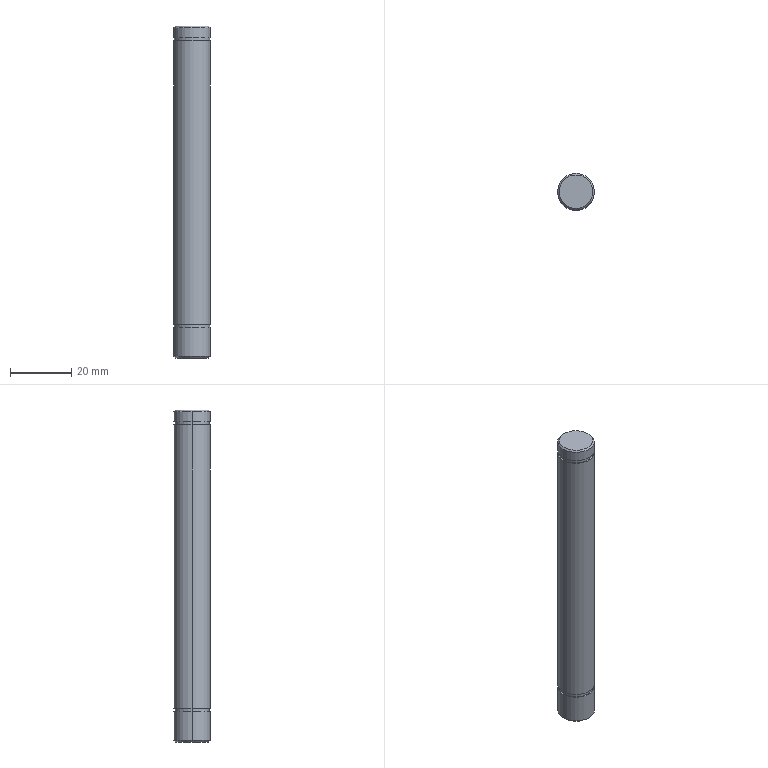Part | STEP file | 2013 Bag feed rotary shaft | 1 solid | 24 faces | box 12 x 12 x 108.5 mm | volume 11898 mm3 | cylinder 12 | cone 6 | plane 6 | commonest cylinder face diameters 12 x6 11.5 x4 5 x2
STEP:
#1=CARTESIAN_POINT('',(0.,0.,0.));
#2=DIRECTION('',(0.,0.,1.));
#3=DIRECTION('',(1.,0.,0.));
#4=AXIS2_PLACEMENT_3D('',#1,#2,#3);
#5=CARTESIAN_POINT('',(-5.5,0.,-11.1));
#6=VERTEX_POINT('',#5);
#7=CARTESIAN_POINT('',(5.5,0.,-11.1));
#8=VERTEX_POINT('',#7);
#9=CARTESIAN_POINT('',(0.,0.,-11.1));
#10=DIRECTION('',(0.,0.,-1.));
#11=DIRECTION('',(-1.,0.,0.));
#12=AXIS2_PLACEMENT_3D('',#9,#10,#11);
#13=CIRCLE('',#12,5.5);
#14=CARTESIAN_POINT('',(0.,0.,-11.1));
#15=DIRECTION('',(0.,0.,1.));
#16=DIRECTION('',(1.,0.,0.));
#17=AXIS2_PLACEMENT_3D('',#14,#15,#16);
#18=CONICAL_SURFACE('',#17,5.5,0.7854);
#19=CARTESIAN_POINT('',(3.142,0.));
#20=DIRECTION('',(-1.,0.));
#21=VECTOR('',#20,1.);
#22=LINE('',#19,#21);
#23=(GEOMETRIC_REPRESENTATION_CONTEXT(2)PARAMETRIC_REPRESENTATION_CONTEXT()REPRESENTATION_CONTEXT('',''));
#24=DEFINITIONAL_REPRESENTATION('',(#22),#23);
#25=PCURVE('',#18,#24);
#26=CARTESIAN_POINT('',(0.,0.,-11.1));
#27=DIRECTION('',(0.,0.,-1.));
#28=DIRECTION('',(-1.,0.,0.));
#29=AXIS2_PLACEMENT_3D('',#26,#27,#28);
#30=PLANE('',#29);
#31=CARTESIAN_POINT('',(0.,0.));
#32=DIRECTION('',(1.,0.));
#33=AXIS2_PLACEMENT_2D('',#31,#32);
#34=CIRCLE('',#33,5.5);
#35=(GEOMETRIC_REPRESENTATION_CONTEXT(2)PARAMETRIC_REPRESENTATION_CONTEXT()REPRESENTATION_CONTEXT('',''));
#36=DEFINITIONAL_REPRESENTATION('',(#34),#35);
#37=PCURVE('',#30,#36);
#38=SURFACE_CURVE('',#13,(#25,#37),.PCURVE_S1.);
#39=EDGE_CURVE('',#6,#8,#38,.T.);
#40=ORIENTED_EDGE('',*,*,#39,.F.);
#41=CARTESIAN_POINT('',(-6.,0.,-10.6));
#42=VERTEX_POINT('',#41);
#43=CARTESIAN_POINT('',(-5.5,0.,-11.1));
#44=DIRECTION('',(-0.7071,0.,0.7071));
#45=VECTOR('',#44,1.);
#46=LINE('',#43,#45);
#47=CARTESIAN_POINT('',(3.142,0.));
#48=DIRECTION('',(0.,1.));
#49=VECTOR('',#48,1.);
#50=LINE('',#47,#49);
#51=(GEOMETRIC_REPRESENTATION_CONTEXT(2)PARAMETRIC_REPRESENTATION_CONTEXT()REPRESENTATION_CONTEXT('',''));
#52=DEFINITIONAL_REPRESENTATION('',(#50),#51);
#53=PCURVE('',#18,#52);
#54=CARTESIAN_POINT('',(0.,0.,-11.1));
#55=DIRECTION('',(0.,0.,1.));
#56=DIRECTION('',(1.,0.,0.));
#57=AXIS2_PLACEMENT_3D('',#54,#55,#56);
#58=CONICAL_SURFACE('',#57,5.5,0.7854);
#59=CARTESIAN_POINT('',(3.142,0.));
#60=DIRECTION('',(0.,1.));
#61=VECTOR('',#60,1.);
#62=LINE('',#59,#61);
#63=(GEOMETRIC_REPRESENTATION_CONTEXT(2)PARAMETRIC_REPRESENTATION_CONTEXT()REPRESENTATION_CONTEXT('',''));
#64=DEFINITIONAL_REPRESENTATION('',(#62),#63);
#65=PCURVE('',#58,#64);
#66=SURFACE_CURVE('',#46,(#53,#65),.PCURVE_S1.);
#67=EDGE_CURVE('',#6,#42,#66,.T.);
#68=ORIENTED_EDGE('',*,*,#67,.T.);
#69=CARTESIAN_POINT('',(6.,0.,-10.6));
#70=VERTEX_POINT('',#69);
#71=CARTESIAN_POINT('',(0.,0.,-10.6));
#72=DIRECTION('',(0.,0.,1.));
#73=DIRECTION('',(-1.,0.,0.));
#74=AXIS2_PLACEMENT_3D('',#71,#72,#73);
#75=CIRCLE('',#74,6.);
#76=CARTESIAN_POINT('',(-3.142,0.5));
#77=DIRECTION('',(1.,0.));
#78=VECTOR('',#77,1.);
#79=LINE('',#76,#78);
#80=(GEOMETRIC_REPRESENTATION_CONTEXT(2)PARAMETRIC_REPRESENTATION_CONTEXT()REPRESENTATION_CONTEXT('',''));
#81=DEFINITIONAL_REPRESENTATION('',(#79),#80);
#82=PCURVE('',#18,#81);
#83=CARTESIAN_POINT('',(0.,0.,-11.1));
#84=DIRECTION('',(0.,0.,1.));
#85=DIRECTION('',(1.,0.,0.));
#86=AXIS2_PLACEMENT_3D('',#83,#84,#85);
#87=CYLINDRICAL_SURFACE('',#86,6.);
#88=CARTESIAN_POINT('',(-3.142,0.5));
#89=DIRECTION('',(1.,0.));
#90=VECTOR('',#89,1.);
#91=LINE('',#88,#90);
#92=(GEOMETRIC_REPRESENTATION_CONTEXT(2)PARAMETRIC_REPRESENTATION_CONTEXT()REPRESENTATION_CONTEXT('',''));
#93=DEFINITIONAL_REPRESENTATION('',(#91),#92);
#94=PCURVE('',#87,#93);
#95=SURFACE_CURVE('',#75,(#82,#94),.PCURVE_S1.);
#96=EDGE_CURVE('',#70,#42,#95,.T.);
#97=ORIENTED_EDGE('',*,*,#96,.F.);
#98=CARTESIAN_POINT('',(5.5,0.,-11.1));
#99=DIRECTION('',(0.7071,0.,0.7071));
#100=VECTOR('',#99,1.);
#101=LINE('',#98,#100);
#102=CARTESIAN_POINT('',(0.,0.));
#103=DIRECTION('',(0.,1.));
#104=VECTOR('',#103,1.);
#105=LINE('',#102,#104);
#106=(GEOMETRIC_REPRESENTATION_CONTEXT(2)PARAMETRIC_REPRESENTATION_CONTEXT()REPRESENTATION_CONTEXT('',''));
#107=DEFINITIONAL_REPRESENTATION('',(#105),#106);
#108=PCURVE('',#18,#107);
#109=CARTESIAN_POINT('',(6.283,0.));
#110=DIRECTION('',(0.,1.));
#111=VECTOR('',#110,1.);
#112=LINE('',#109,#111);
#113=(GEOMETRIC_REPRESENTATION_CONTEXT(2)PARAMETRIC_REPRESENTATION_CONTEXT()REPRESENTATION_CONTEXT('',''));
#114=DEFINITIONAL_REPRESENTATION('',(#112),#113);
#115=PCURVE('',#58,#114);
#116=SURFACE_CURVE('',#101,(#108,#115),.PCURVE_S1.);
#117=EDGE_CURVE('',#8,#70,#116,.T.);
#118=ORIENTED_EDGE('',*,*,#117,.F.);
#119=EDGE_LOOP('',(#40,#68,#97,#118));
#120=FACE_BOUND('',#119,.T.);
#121=ADVANCED_FACE('',(#120),#18,.T.);
#122=CARTESIAN_POINT('',(5.5,0.,97.4));
#123=VERTEX_POINT('',#122);
#124=CARTESIAN_POINT('',(-5.5,0.,97.4));
#125=VERTEX_POINT('',#124);
#126=CARTESIAN_POINT('',(0.,0.,97.4));
#127=DIRECTION('',(0.,0.,1.));
#128=DIRECTION('',(1.,0.,0.));
#129=AXIS2_PLACEMENT_3D('',#126,#127,#128);
#130=CIRCLE('',#129,5.5);
#131=CARTESIAN_POINT('',(0.,0.,97.4));
#132=DIRECTION('',(0.,0.,-1.));
#133=DIRECTION('',(-1.,0.,0.));
#134=AXIS2_PLACEMENT_3D('',#131,#132,#133);
#135=CONICAL_SURFACE('',#134,5.5,0.7854);
#136=CARTESIAN_POINT('',(3.142,0.));
#137=DIRECTION('',(-1.,0.));
#138=VECTOR('',#137,1.);
#139=LINE('',#136,#138);
#140=(GEOMETRIC_REPRESENTATION_CONTEXT(2)PARAMETRIC_REPRESENTATION_CONTEXT()REPRESENTATION_CONTEXT('',''));
#141=DEFINITIONAL_REPRESENTATION('',(#139),#140);
#142=PCURVE('',#135,#141);
#143=CARTESIAN_POINT('',(0.,0.,97.4));
#144=DIRECTION('',(0.,0.,1.));
#145=DIRECTION('',(1.,0.,0.));
#146=AXIS2_PLACEMENT_3D('',#143,#144,#145);
#147=PLANE('',#146);
#148=CARTESIAN_POINT('',(0.,0.));
#149=DIRECTION('',(1.,0.));
#150=AXIS2_PLACEMENT_2D('',#148,#149);
#151=CIRCLE('',#150,5.5);
#152=(GEOMETRIC_REPRESENTATION_CONTEXT(2)PARAMETRIC_REPRESENTATION_CONTEXT()REPRESENTATION_CONTEXT('',''));
#153=DEFINITIONAL_REPRESENTATION('',(#151),#152);
#154=PCURVE('',#147,#153);
#155=SURFACE_CURVE('',#130,(#142,#154),.PCURVE_S1.);
#156=EDGE_CURVE('',#123,#125,#155,.T.);
#157=ORIENTED_EDGE('',*,*,#156,.F.);
#158=CARTESIAN_POINT('',(6.,0.,96.9));
#159=VERTEX_POINT('',#158);
#160=CARTESIAN_POINT('',(5.5,0.,97.4));
#161=DIRECTION('',(0.7071,0.,-0.7071));
#162=VECTOR('',#161,1.);
#163=LINE('',#160,#162);
#164=CARTESIAN_POINT('',(3.142,0.));
#165=DIRECTION('',(0.,1.));
#166=VECTOR('',#165,1.);
#167=LINE('',#164,#166);
#168=(GEOMETRIC_REPRESENTATION_CONTEXT(2)PARAMETRIC_REPRESENTATION_CONTEXT()REPRESENTATION_CONTEXT('',''));
#169=DEFINITIONAL_REPRESENTATION('',(#167),#168);
#170=PCURVE('',#135,#169);
#171=CARTESIAN_POINT('',(0.,0.,97.4));
#172=DIRECTION('',(0.,0.,-1.));
#173=DIRECTION('',(-1.,0.,0.));
#174=AXIS2_PLACEMENT_3D('',#171,#172,#173);
#175=CONICAL_SURFACE('',#174,5.5,0.7854);
#176=CARTESIAN_POINT('',(3.142,0.));
#177=DIRECTION('',(0.,1.));
#178=VECTOR('',#177,1.);
#179=LINE('',#176,#178);
#180=(GEOMETRIC_REPRESENTATION_CONTEXT(2)PARAMETRIC_REPRESENTATION_CONTEXT()REPRESENTATION_CONTEXT('',''));
#181=DEFINITIONAL_REPRESENTATION('',(#179),#180);
#182=PCURVE('',#175,#181);
#183=SURFACE_CURVE('',#163,(#170,#182),.PCURVE_S1.);
#184=EDGE_CURVE('',#123,#159,#183,.T.);
#185=ORIENTED_EDGE('',*,*,#184,.T.);
#186=CARTESIAN_POINT('',(-6.,0.,96.9));
#187=VERTEX_POINT('',#186);
#188=CARTESIAN_POINT('',(0.,0.,96.9));
#189=DIRECTION('',(0.,0.,-1.));
#190=DIRECTION('',(1.,0.,0.));
#191=AXIS2_PLACEMENT_3D('',#188,#189,#190);
#192=CIRCLE('',#191,6.);
#193=CARTESIAN_POINT('',(-3.142,0.5));
#194=DIRECTION('',(1.,0.));
#195=VECTOR('',#194,1.);
#196=LINE('',#193,#195);
#197=(GEOMETRIC_REPRESENTATION_CONTEXT(2)PARAMETRIC_REPRESENTATION_CONTEXT()REPRESENTATION_CONTEXT('',''));
#198=DEFINITIONAL_REPRESENTATION('',(#196),#197);
#199=PCURVE('',#135,#198);
#200=CARTESIAN_POINT('',(0.,0.,97.4));
#201=DIRECTION('',(0.,0.,-1.));
#202=DIRECTION('',(-1.,0.,0.));
#203=AXIS2_PLACEMENT_3D('',#200,#201,#202);
#204=CYLINDRICAL_SURFACE('',#203,6.);
#205=CARTESIAN_POINT('',(-3.142,0.5));
#206=DIRECTION('',(1.,0.));
#207=VECTOR('',#206,1.);
#208=LINE('',#205,#207);
#209=(GEOMETRIC_REPRESENTATION_CONTEXT(2)PARAMETRIC_REPRESENTATION_CONTEXT()REPRESENTATION_CONTEXT('',''));
#210=DEFINITIONAL_REPRESENTATION('',(#208),#209);
#211=PCURVE('',#204,#210);
#212=SURFACE_CURVE('',#192,(#199,#211),.PCURVE_S1.);
#213=EDGE_CURVE('',#187,#159,#212,.T.);
#214=ORIENTED_EDGE('',*,*,#213,.F.);
#215=CARTESIAN_POINT('',(-5.5,0.,97.4));
#216=DIRECTION('',(-0.7071,0.,-0.7071));
#217=VECTOR('',#216,1.);
#218=LINE('',#215,#217);
#219=CARTESIAN_POINT('',(0.,0.));
#220=DIRECTION('',(0.,1.));
#221=VECTOR('',#220,1.);
#222=LINE('',#219,#221);
#223=(GEOMETRIC_REPRESENTATION_CONTEXT(2)PARAMETRIC_REPRESENTATION_CONTEXT()REPRESENTATION_CONTEXT('',''));
#224=DEFINITIONAL_REPRESENTATION('',(#222),#223);
#225=PCURVE('',#135,#224);
#226=CARTESIAN_POINT('',(6.283,0.));
#227=DIRECTION('',(0.,1.));
#228=VECTOR('',#227,1.);
#229=LINE('',#226,#228);
#230=(GEOMETRIC_REPRESENTATION_CONTEXT(2)PARAMETRIC_REPRESENTATION_CONTEXT()REPRESENTATION_CONTEXT('',''));
#231=DEFINITIONAL_REPRESENTATION('',(#229),#230);
#232=PCURVE('',#175,#231);
#233=SURFACE_CURVE('',#218,(#225,#232),.PCURVE_S1.);
#234=EDGE_CURVE('',#125,#187,#233,.T.);
#235=ORIENTED_EDGE('',*,*,#234,.F.);
#236=EDGE_LOOP('',(#157,#185,#214,#235));
#237=FACE_BOUND('',#236,.T.);
#238=ADVANCED_FACE('',(#237),#135,.T.);
#239=CARTESIAN_POINT('',(-2.5,0.,5.9));
#240=VERTEX_POINT('',#239);
#241=CARTESIAN_POINT('',(-2.5,0.,-11.1));
#242=VERTEX_POINT('',#241);
#243=CARTESIAN_POINT('',(-2.5,0.,-11.1));
#244=DIRECTION('',(0.,0.,-1.));
#245=VECTOR('',#244,1.);
#246=LINE('',#243,#245);
#247=CARTESIAN_POINT('',(0.,0.,-11.1));
#248=DIRECTION('',(0.,0.,-1.));
#249=DIRECTION('',(-1.,0.,0.));
#250=AXIS2_PLACEMENT_3D('',#247,#248,#249);
#251=CYLINDRICAL_SURFACE('',#250,2.5);
#252=CARTESIAN_POINT('',(6.283,0.));
#253=DIRECTION('',(0.,1.));
#254=VECTOR('',#253,1.);
#255=LINE('',#252,#254);
#256=(GEOMETRIC_REPRESENTATION_CONTEXT(2)PARAMETRIC_REPRESENTATION_CONTEXT()REPRESENTATION_CONTEXT('',''));
#257=DEFINITIONAL_REPRESENTATION('',(#255),#256);
#258=PCURVE('',#251,#257);
#259=CARTESIAN_POINT('',(0.,0.,-11.1));
#260=DIRECTION('',(0.,0.,-1.));
#261=DIRECTION('',(-1.,0.,0.));
#262=AXIS2_PLACEMENT_3D('',#259,#260,#261);
#263=CYLINDRICAL_SURFACE('',#262,2.5);
#264=CARTESIAN_POINT('',(0.,0.));
#265=DIRECTION('',(0.,1.));
#266=VECTOR('',#265,1.);
#267=LINE('',#264,#266);
#268=(GEOMETRIC_REPRESENTATION_CONTEXT(2)PARAMETRIC_REPRESENTATION_CONTEXT()REPRESENTATION_CONTEXT('',''));
#269=DEFINITIONAL_REPRESENTATION('',(#267),#268);
#270=PCURVE('',#263,#269);
#271=SURFACE_CURVE('',#246,(#258,#270),.PCURVE_S1.);
#272=EDGE_CURVE('',#240,#242,#271,.T.);
#273=ORIENTED_EDGE('',*,*,#272,.T.);
#274=CARTESIAN_POINT('',(2.5,0.,-11.1));
#275=VERTEX_POINT('',#274);
#276=CARTESIAN_POINT('',(0.,0.,-11.1));
#277=DIRECTION('',(0.,0.,-1.));
#278=DIRECTION('',(-1.,0.,0.));
#279=AXIS2_PLACEMENT_3D('',#276,#277,#278);
#280=CIRCLE('',#279,2.5);
#281=CARTESIAN_POINT('',(0.,0.));
#282=DIRECTION('',(1.,0.));
#283=VECTOR('',#282,1.);
#284=LINE('',#281,#283);
#285=(GEOMETRIC_REPRESENTATION_CONTEXT(2)PARAMETRIC_REPRESENTATION_CONTEXT()REPRESENTATION_CONTEXT('',''));
#286=DEFINITIONAL_REPRESENTATION('',(#284),#285);
#287=PCURVE('',#251,#286);
#288=CARTESIAN_POINT('',(0.,0.));
#289=DIRECTION('',(1.,0.));
#290=AXIS2_PLACEMENT_2D('',#288,#289);
#291=CIRCLE('',#290,2.5);
#292=(GEOMETRIC_REPRESENTATION_CONTEXT(2)PARAMETRIC_REPRESENTATION_CONTEXT()REPRESENTATION_CONTEXT('',''));
#293=DEFINITIONAL_REPRESENTATION('',(#291),#292);
#294=PCURVE('',#30,#293);
#295=SURFACE_CURVE('',#280,(#287,#294),.PCURVE_S1.);
#296=EDGE_CURVE('',#275,#242,#295,.T.);
#297=ORIENTED_EDGE('',*,*,#296,.F.);
#298=CARTESIAN_POINT('',(2.5,0.,5.9));
#299=VERTEX_POINT('',#298);
#300=CARTESIAN_POINT('',(2.5,0.,-11.1));
#301=DIRECTION('',(0.,0.,-1.));
#302=VECTOR('',#301,1.);
#303=LINE('',#300,#302);
#304=CARTESIAN_POINT('',(3.142,0.));
#305=DIRECTION('',(0.,1.));
#306=VECTOR('',#305,1.);
#307=LINE('',#304,#306);
#308=(GEOMETRIC_REPRESENTATION_CONTEXT(2)PARAMETRIC_REPRESENTATION_CONTEXT()REPRESENTATION_CONTEXT('',''));
#309=DEFINITIONAL_REPRESENTATION('',(#307),#308);
#310=PCURVE('',#251,#309);
#311=CARTESIAN_POINT('',(3.142,0.));
#312=DIRECTION('',(0.,1.));
#313=VECTOR('',#312,1.);
#314=LINE('',#311,#313);
#315=(GEOMETRIC_REPRESENTATION_CONTEXT(2)PARAMETRIC_REPRESENTATION_CONTEXT()REPRESENTATION_CONTEXT('',''));
#316=DEFINITIONAL_REPRESENTATION('',(#314),#315);
#317=PCURVE('',#263,#316);
#318=SURFACE_CURVE('',#303,(#310,#317),.PCURVE_S1.);
#319=EDGE_CURVE('',#299,#275,#318,.T.);
#320=ORIENTED_EDGE('',*,*,#319,.F.);
#321=CARTESIAN_POINT('',(0.,0.,5.9));
#322=DIRECTION('',(0.,0.,-1.));
#323=DIRECTION('',(-1.,0.,0.));
#324=AXIS2_PLACEMENT_3D('',#321,#322,#323);
#325=CIRCLE('',#324,2.5);
#326=CARTESIAN_POINT('',(0.,-17.));
#327=DIRECTION('',(1.,0.));
#328=VECTOR('',#327,1.);
#329=LINE('',#326,#328);
#330=(GEOMETRIC_REPRESENTATION_CONTEXT(2)PARAMETRIC_REPRESENTATION_CONTEXT()REPRESENTATION_CONTEXT('',''));
#331=DEFINITIONAL_REPRESENTATION('',(#329),#330);
#332=PCURVE('',#251,#331);
#333=CARTESIAN_POINT('',(0.,0.,5.9));
#334=DIRECTION('',(0.,0.,-1.));
#335=DIRECTION('',(-1.,0.,0.));
#336=AXIS2_PLACEMENT_3D('',#333,#334,#335);
#337=CONICAL_SURFACE('',#336,2.5,1.03);
#338=CARTESIAN_POINT('',(0.,0.));
#339=DIRECTION('',(1.,0.));
#340=VECTOR('',#339,1.);
#341=LINE('',#338,#340);
#342=(GEOMETRIC_REPRESENTATION_CONTEXT(2)PARAMETRIC_REPRESENTATION_CONTEXT()REPRESENTATION_CONTEXT('',''));
#343=DEFINITIONAL_REPRESENTATION('',(#341),#342);
#344=PCURVE('',#337,#343);
#345=SURFACE_CURVE('',#325,(#332,#344),.PCURVE_S1.);
#346=EDGE_CURVE('',#299,#240,#345,.T.);
#347=ORIENTED_EDGE('',*,*,#346,.T.);
#348=EDGE_LOOP('',(#273,#297,#320,#347));
#349=FACE_BOUND('',#348,.F.);
#350=ADVANCED_FACE('',(#349),#251,.F.);
#351=ORIENTED_EDGE('',*,*,#346,.F.);
#352=CARTESIAN_POINT('',(0.,0.,7.402));
#353=VERTEX_POINT('',#352);
#354=CARTESIAN_POINT('',(2.5,0.,5.9));
#355=DIRECTION('',(0.8572,0.,-0.515));
#356=VECTOR('',#355,1.);
#357=LINE('',#354,#356);
#358=CARTESIAN_POINT('',(3.142,0.));
#359=DIRECTION('',(0.,1.));
#360=VECTOR('',#359,1.);
#361=LINE('',#358,#360);
#362=(GEOMETRIC_REPRESENTATION_CONTEXT(2)PARAMETRIC_REPRESENTATION_CONTEXT()REPRESENTATION_CONTEXT('',''));
#363=DEFINITIONAL_REPRESENTATION('',(#361),#362);
#364=PCURVE('',#337,#363);
#365=CARTESIAN_POINT('',(0.,0.,5.9));
#366=DIRECTION('',(0.,0.,-1.));
#367=DIRECTION('',(-1.,0.,0.));
#368=AXIS2_PLACEMENT_3D('',#365,#366,#367);
#369=CONICAL_SURFACE('',#368,2.5,1.03);
#370=CARTESIAN_POINT('',(3.142,0.));
#371=DIRECTION('',(0.,1.));
#372=VECTOR('',#371,1.);
#373=LINE('',#370,#372);
#374=(GEOMETRIC_REPRESENTATION_CONTEXT(2)PARAMETRIC_REPRESENTATION_CONTEXT()REPRESENTATION_CONTEXT('',''));
#375=DEFINITIONAL_REPRESENTATION('',(#373),#374);
#376=PCURVE('',#369,#375);
#377=SURFACE_CURVE('',#357,(#364,#376),.PCURVE_S1.);
#378=EDGE_CURVE('',#353,#299,#377,.T.);
#379=ORIENTED_EDGE('',*,*,#378,.F.);
#380=CARTESIAN_POINT('',(-2.5,0.,5.9));
#381=DIRECTION('',(-0.8572,0.,-0.515));
#382=VECTOR('',#381,1.);
#383=LINE('',#380,#382);
#384=CARTESIAN_POINT('',(6.283,0.));
#385=DIRECTION('',(0.,1.));
#386=VECTOR('',#385,1.);
#387=LINE('',#384,#386);
#388=(GEOMETRIC_REPRESENTATION_CONTEXT(2)PARAMETRIC_REPRESENTATION_CONTEXT()REPRESENTATION_CONTEXT('',''));
#389=DEFINITIONAL_REPRESENTATION('',(#387),#388);
#390=PCURVE('',#337,#389);
#391=CARTESIAN_POINT('',(0.,0.));
#392=DIRECTION('',(0.,1.));
#393=VECTOR('',#392,1.);
#394=LINE('',#391,#393);
#395=(GEOMETRIC_REPRESENTATION_CONTEXT(2)PARAMETRIC_REPRESENTATION_CONTEXT()REPRESENTATION_CONTEXT('',''));
#396=DEFINITIONAL_REPRESENTATION('',(#394),#395);
#397=PCURVE('',#369,#396);
#398=SURFACE_CURVE('',#383,(#390,#397),.PCURVE_S1.);
#399=EDGE_CURVE('',#353,#240,#398,.T.);
#400=ORIENTED_EDGE('',*,*,#399,.T.);
#401=EDGE_LOOP('',(#351,#379,#400));
#402=FACE_BOUND('',#401,.F.);
#403=ADVANCED_FACE('',(#402),#337,.F.);
#404=ORIENTED_EDGE('',*,*,#96,.T.);
#405=CARTESIAN_POINT('',(-6.,0.,-1.1));
#406=VERTEX_POINT('',#405);
#407=CARTESIAN_POINT('',(-6.,0.,-11.1));
#408=DIRECTION('',(0.,0.,1.));
#409=VECTOR('',#408,1.);
#410=LINE('',#407,#409);
#411=CARTESIAN_POINT('',(3.142,0.));
#412=DIRECTION('',(0.,1.));
#413=VECTOR('',#412,1.);
#414=LINE('',#411,#413);
#415=(GEOMETRIC_REPRESENTATION_CONTEXT(2)PARAMETRIC_REPRESENTATION_CONTEXT()REPRESENTATION_CONTEXT('',''));
#416=DEFINITIONAL_REPRESENTATION('',(#414),#415);
#417=PCURVE('',#87,#416);
#418=CARTESIAN_POINT('',(0.,0.,-11.1));
#419=DIRECTION('',(0.,0.,1.));
#420=DIRECTION('',(1.,0.,0.));
#421=AXIS2_PLACEMENT_3D('',#418,#419,#420);
#422=CYLINDRICAL_SURFACE('',#421,6.);
#423=CARTESIAN_POINT('',(3.142,0.));
#424=DIRECTION('',(0.,1.));
#425=VECTOR('',#424,1.);
#426=LINE('',#423,#425);
#427=(GEOMETRIC_REPRESENTATION_CONTEXT(2)PARAMETRIC_REPRESENTATION_CONTEXT()REPRESENTATION_CONTEXT('',''));
#428=DEFINITIONAL_REPRESENTATION('',(#426),#427);
#429=PCURVE('',#422,#428);
#430=SURFACE_CURVE('',#410,(#417,#429),.PCURVE_S1.);
#431=EDGE_CURVE('',#42,#406,#430,.T.);
#432=ORIENTED_EDGE('',*,*,#431,.T.);
#433=CARTESIAN_POINT('',(6.,0.,-1.1));
#434=VERTEX_POINT('',#433);
#435=CARTESIAN_POINT('',(0.,0.,-1.1));
#436=DIRECTION('',(0.,0.,-1.));
#437=DIRECTION('',(-1.,0.,0.));
#438=AXIS2_PLACEMENT_3D('',#435,#436,#437);
#439=CIRCLE('',#438,6.);
#440=CARTESIAN_POINT('',(3.142,10.));
#441=DIRECTION('',(-1.,0.));
#442=VECTOR('',#441,1.);
#443=LINE('',#440,#442);
#444=(GEOMETRIC_REPRESENTATION_CONTEXT(2)PARAMETRIC_REPRESENTATION_CONTEXT()REPRESENTATION_CONTEXT('',''));
#445=DEFINITIONAL_REPRESENTATION('',(#443),#444);
#446=PCURVE('',#87,#445);
#447=CARTESIAN_POINT('',(0.,0.,-1.1));
#448=DIRECTION('',(0.,0.,-1.));
#449=DIRECTION('',(-1.,0.,0.));
#450=AXIS2_PLACEMENT_3D('',#447,#448,#449);
#451=PLANE('',#450);
#452=CARTESIAN_POINT('',(0.,0.));
#453=DIRECTION('',(1.,0.));
#454=AXIS2_PLACEMENT_2D('',#452,#453);
#455=CIRCLE('',#454,6.);
#456=(GEOMETRIC_REPRESENTATION_CONTEXT(2)PARAMETRIC_REPRESENTATION_CONTEXT()REPRESENTATION_CONTEXT('',''));
#457=DEFINITIONAL_REPRESENTATION('',(#455),#456);
#458=PCURVE('',#451,#457);
#459=SURFACE_CURVE('',#439,(#446,#458),.PCURVE_S1.);
#460=EDGE_CURVE('',#406,#434,#459,.T.);
#461=ORIENTED_EDGE('',*,*,#460,.T.);
#462=CARTESIAN_POINT('',(6.,0.,-11.1));
#463=DIRECTION('',(0.,0.,1.));
#464=VECTOR('',#463,1.);
#465=LINE('',#462,#464);
#466=CARTESIAN_POINT('',(0.,0.));
#467=DIRECTION('',(0.,1.));
#468=VECTOR('',#467,1.);
#469=LINE('',#466,#468);
#470=(GEOMETRIC_REPRESENTATION_CONTEXT(2)PARAMETRIC_REPRESENTATION_CONTEXT()REPRESENTATION_CONTEXT('',''));
#471=DEFINITIONAL_REPRESENTATION('',(#469),#470);
#472=PCURVE('',#87,#471);
#473=CARTESIAN_POINT('',(6.283,0.));
#474=DIRECTION('',(0.,1.));
#475=VECTOR('',#474,1.);
#476=LINE('',#473,#475);
#477=(GEOMETRIC_REPRESENTATION_CONTEXT(2)PARAMETRIC_REPRESENTATION_CONTEXT()REPRESENTATION_CONTEXT('',''));
#478=DEFINITIONAL_REPRESENTATION('',(#476),#477);
#479=PCURVE('',#422,#478);
#480=SURFACE_CURVE('',#465,(#472,#479),.PCURVE_S1.);
#481=EDGE_CURVE('',#70,#434,#480,.T.);
#482=ORIENTED_EDGE('',*,*,#481,.F.);
#483=EDGE_LOOP('',(#404,#432,#461,#482));
#484=FACE_BOUND('',#483,.T.);
#485=ADVANCED_FACE('',(#484),#87,.T.);
#486=CARTESIAN_POINT('',(-5.75,0.,-1.1));
#487=VERTEX_POINT('',#486);
#488=CARTESIAN_POINT('',(5.75,0.,-1.1));
#489=VERTEX_POINT('',#488);
#490=CARTESIAN_POINT('',(0.,0.,-1.1));
#491=DIRECTION('',(0.,0.,-1.));
#492=DIRECTION('',(-1.,0.,0.));
#493=AXIS2_PLACEMENT_3D('',#490,#491,#492);
#494=CIRCLE('',#493,5.75);
#495=CARTESIAN_POINT('',(0.,0.,-1.1));
#496=DIRECTION('',(0.,0.,1.));
#497=DIRECTION('',(1.,0.,0.));
#498=AXIS2_PLACEMENT_3D('',#495,#496,#497);
#499=CYLINDRICAL_SURFACE('',#498,5.75);
#500=CARTESIAN_POINT('',(3.142,0.));
#501=DIRECTION('',(-1.,0.));
#502=VECTOR('',#501,1.);
#503=LINE('',#500,#502);
#504=(GEOMETRIC_REPRESENTATION_CONTEXT(2)PARAMETRIC_REPRESENTATION_CONTEXT()REPRESENTATION_CONTEXT('',''));
#505=DEFINITIONAL_REPRESENTATION('',(#503),#504);
#506=PCURVE('',#499,#505);
#507=CARTESIAN_POINT('',(0.,0.));
#508=DIRECTION('',(1.,0.));
#509=AXIS2_PLACEMENT_2D('',#507,#508);
#510=CIRCLE('',#509,5.75);
#511=(GEOMETRIC_REPRESENTATION_CONTEXT(2)PARAMETRIC_REPRESENTATION_CONTEXT()REPRESENTATION_CONTEXT('',''));
#512=DEFINITIONAL_REPRESENTATION('',(#510),#511);
#513=PCURVE('',#451,#512);
#514=SURFACE_CURVE('',#494,(#506,#513),.PCURVE_S1.);
#515=EDGE_CURVE('',#487,#489,#514,.T.);
#516=ORIENTED_EDGE('',*,*,#515,.F.);
#517=CARTESIAN_POINT('',(-5.75,0.,0.));
#518=VERTEX_POINT('',#517);
#519=CARTESIAN_POINT('',(-5.75,0.,-1.1));
#520=DIRECTION('',(0.,0.,1.));
#521=VECTOR('',#520,1.);
#522=LINE('',#519,#521);
#523=CARTESIAN_POINT('',(3.142,0.));
#524=DIRECTION('',(0.,1.));
#525=VECTOR('',#524,1.);
#526=LINE('',#523,#525);
#527=(GEOMETRIC_REPRESENTATION_CONTEXT(2)PARAMETRIC_REPRESENTATION_CONTEXT()REPRESENTATION_CONTEXT('',''));
#528=DEFINITIONAL_REPRESENTATION('',(#526),#527);
#529=PCURVE('',#499,#528);
#530=CARTESIAN_POINT('',(0.,0.,-1.1));
#531=DIRECTION('',(0.,0.,1.));
#532=DIRECTION('',(1.,0.,0.));
#533=AXIS2_PLACEMENT_3D('',#530,#531,#532);
#534=CYLINDRICAL_SURFACE('',#533,5.75);
#535=CARTESIAN_POINT('',(3.142,0.));
#536=DIRECTION('',(0.,1.));
#537=VECTOR('',#536,1.);
#538=LINE('',#535,#537);
#539=(GEOMETRIC_REPRESENTATION_CONTEXT(2)PARAMETRIC_REPRESENTATION_CONTEXT()REPRESENTATION_CONTEXT('',''));
#540=DEFINITIONAL_REPRESENTATION('',(#538),#539);
#541=PCURVE('',#534,#540);
#542=SURFACE_CURVE('',#522,(#529,#541),.PCURVE_S1.);
#543=EDGE_CURVE('',#487,#518,#542,.T.);
#544=ORIENTED_EDGE('',*,*,#543,.T.);
#545=CARTESIAN_POINT('',(5.75,0.,0.));
#546=VERTEX_POINT('',#545);
#547=CARTESIAN_POINT('',(0.,0.,0.));
#548=DIRECTION('',(0.,0.,-1.));
#549=DIRECTION('',(1.,0.,0.));
#550=AXIS2_PLACEMENT_3D('',#547,#548,#549);
#551=CIRCLE('',#550,5.75);
#552=CARTESIAN_POINT('',(6.283,1.1));
#553=DIRECTION('',(-1.,0.));
#554=VECTOR('',#553,1.);
#555=LINE('',#552,#554);
#556=(GEOMETRIC_REPRESENTATION_CONTEXT(2)PARAMETRIC_REPRESENTATION_CONTEXT()REPRESENTATION_CONTEXT('',''));
#557=DEFINITIONAL_REPRESENTATION('',(#555),#556);
#558=PCURVE('',#499,#557);
#559=CARTESIAN_POINT('',(0.,0.,0.));
#560=DIRECTION('',(0.,0.,1.));
#561=DIRECTION('',(1.,0.,0.));
#562=AXIS2_PLACEMENT_3D('',#559,#560,#561);
#563=PLANE('',#562);
#564=CARTESIAN_POINT('',(5.75,0.));
#565=CARTESIAN_POINT('',(5.75,-9.959));
#566=CARTESIAN_POINT('',(-2.875,-4.98));
#567=CARTESIAN_POINT('',(-11.5,0.));
#568=CARTESIAN_POINT('',(-2.875,4.98));
#569=CARTESIAN_POINT('',(5.75,9.959));
#570=CARTESIAN_POINT('',(5.75,0.));
#571=(BOUNDED_CURVE()B_SPLINE_CURVE(2,(#564,#565,#566,#567,#568,#569,#570),.UNSPECIFIED.,.T.,.F.)B_SPLINE_CURVE_WITH_KNOTS((1,2,2,2,2,1),(-2.094,0.,2.094,4.189,6.283,8.378),.UNSPECIFIED.)CURVE()GEOMETRIC_REPRESENTATION_ITEM()RATIONAL_B_SPLINE_CURVE((1.,0.5,1.,0.5,1.,0.5,1.))REPRESENTATION_ITEM(''));
#572=(GEOMETRIC_REPRESENTATION_CONTEXT(2)PARAMETRIC_REPRESENTATION_CONTEXT()REPRESENTATION_CONTEXT('',''));
#573=DEFINITIONAL_REPRESENTATION('',(#571),#572);
#574=PCURVE('',#563,#573);
#575=SURFACE_CURVE('',#551,(#558,#574),.PCURVE_S1.);
#576=EDGE_CURVE('',#518,#546,#575,.T.);
#577=ORIENTED_EDGE('',*,*,#576,.T.);
#578=CARTESIAN_POINT('',(5.75,0.,-1.1));
#579=DIRECTION('',(0.,0.,1.));
#580=VECTOR('',#579,1.);
#581=LINE('',#578,#580);
#582=CARTESIAN_POINT('',(0.,0.));
#583=DIRECTION('',(0.,1.));
#584=VECTOR('',#583,1.);
#585=LINE('',#582,#584);
#586=(GEOMETRIC_REPRESENTATION_CONTEXT(2)PARAMETRIC_REPRESENTATION_CONTEXT()REPRESENTATION_CONTEXT('',''));
#587=DEFINITIONAL_REPRESENTATION('',(#585),#586);
#588=PCURVE('',#499,#587);
#589=CARTESIAN_POINT('',(6.283,0.));
#590=DIRECTION('',(0.,1.));
#591=VECTOR('',#590,1.);
#592=LINE('',#589,#591);
#593=(GEOMETRIC_REPRESENTATION_CONTEXT(2)PARAMETRIC_REPRESENTATION_CONTEXT()REPRESENTATION_CONTEXT('',''));
#594=DEFINITIONAL_REPRESENTATION('',(#592),#593);
#595=PCURVE('',#534,#594);
#596=SURFACE_CURVE('',#581,(#588,#595),.PCURVE_S1.);
#597=EDGE_CURVE('',#489,#546,#596,.T.);
#598=ORIENTED_EDGE('',*,*,#597,.F.);
#599=EDGE_LOOP('',(#516,#544,#577,#598));
#600=FACE_BOUND('',#599,.T.);
#601=ADVANCED_FACE('',(#600),#499,.T.);
#602=ORIENTED_EDGE('',*,*,#213,.T.);
#603=CARTESIAN_POINT('',(6.,0.,93.6));
#604=VERTEX_POINT('',#603);
#605=CARTESIAN_POINT('',(6.,0.,97.4));
#606=DIRECTION('',(0.,0.,-1.));
#607=VECTOR('',#606,1.);
#608=LINE('',#605,#607);
#609=CARTESIAN_POINT('',(3.142,0.));
#610=DIRECTION('',(0.,1.));
#611=VECTOR('',#610,1.);
#612=LINE('',#609,#611);
#613=(GEOMETRIC_REPRESENTATION_CONTEXT(2)PARAMETRIC_REPRESENTATION_CONTEXT()REPRESENTATION_CONTEXT('',''));
#614=DEFINITIONAL_REPRESENTATION('',(#612),#613);
#615=PCURVE('',#204,#614);
#616=CARTESIAN_POINT('',(0.,0.,97.4));
#617=DIRECTION('',(0.,0.,-1.));
#618=DIRECTION('',(-1.,0.,0.));
#619=AXIS2_PLACEMENT_3D('',#616,#617,#618);
#620=CYLINDRICAL_SURFACE('',#619,6.);
#621=CARTESIAN_POINT('',(3.142,0.));
#622=DIRECTION('',(0.,1.));
#623=VECTOR('',#622,1.);
#624=LINE('',#621,#623);
#625=(GEOMETRIC_REPRESENTATION_CONTEXT(2)PARAMETRIC_REPRESENTATION_CONTEXT()REPRESENTATION_CONTEXT('',''));
#626=DEFINITIONAL_REPRESENTATION('',(#624),#625);
#627=PCURVE('',#620,#626);
#628=SURFACE_CURVE('',#608,(#615,#627),.PCURVE_S1.);
#629=EDGE_CURVE('',#159,#604,#628,.T.);
#630=ORIENTED_EDGE('',*,*,#629,.T.);
#631=CARTESIAN_POINT('',(-6.,0.,93.6));
#632=VERTEX_POINT('',#631);
#633=CARTESIAN_POINT('',(0.,0.,93.6));
#634=DIRECTION('',(0.,0.,1.));
#635=DIRECTION('',(1.,0.,0.));
#636=AXIS2_PLACEMENT_3D('',#633,#634,#635);
#637=CIRCLE('',#636,6.);
#638=CARTESIAN_POINT('',(3.142,3.8));
#639=DIRECTION('',(-1.,0.));
#640=VECTOR('',#639,1.);
#641=LINE('',#638,#640);
#642=(GEOMETRIC_REPRESENTATION_CONTEXT(2)PARAMETRIC_REPRESENTATION_CONTEXT()REPRESENTATION_CONTEXT('',''));
#643=DEFINITIONAL_REPRESENTATION('',(#641),#642);
#644=PCURVE('',#204,#643);
#645=CARTESIAN_POINT('',(0.,0.,93.6));
#646=DIRECTION('',(0.,0.,1.));
#647=DIRECTION('',(1.,0.,0.));
#648=AXIS2_PLACEMENT_3D('',#645,#646,#647);
#649=PLANE('',#648);
#650=CARTESIAN_POINT('',(0.,0.));
#651=DIRECTION('',(1.,0.));
#652=AXIS2_PLACEMENT_2D('',#650,#651);
#653=CIRCLE('',#652,6.);
#654=(GEOMETRIC_REPRESENTATION_CONTEXT(2)PARAMETRIC_REPRESENTATION_CONTEXT()REPRESENTATION_CONTEXT('',''));
#655=DEFINITIONAL_REPRESENTATION('',(#653),#654);
#656=PCURVE('',#649,#655);
#657=SURFACE_CURVE('',#637,(#644,#656),.PCURVE_S1.);
#658=EDGE_CURVE('',#604,#632,#657,.T.);
#659=ORIENTED_EDGE('',*,*,#658,.T.);
#660=CARTESIAN_POINT('',(-6.,0.,97.4));
#661=DIRECTION('',(0.,0.,-1.));
#662=VECTOR('',#661,1.);
#663=LINE('',#660,#662);
#664=CARTESIAN_POINT('',(0.,0.));
#665=DIRECTION('',(0.,1.));
#666=VECTOR('',#665,1.);
#667=LINE('',#664,#666);
#668=(GEOMETRIC_REPRESENTATION_CONTEXT(2)PARAMETRIC_REPRESENTATION_CONTEXT()REPRESENTATION_CONTEXT('',''));
#669=DEFINITIONAL_REPRESENTATION('',(#667),#668);
#670=PCURVE('',#204,#669);
#671=CARTESIAN_POINT('',(6.283,0.));
#672=DIRECTION('',(0.,1.));
#673=VECTOR('',#672,1.);
#674=LINE('',#671,#673);
#675=(GEOMETRIC_REPRESENTATION_CONTEXT(2)PARAMETRIC_REPRESENTATION_CONTEXT()REPRESENTATION_CONTEXT('',''));
#676=DEFINITIONAL_REPRESENTATION('',(#674),#675);
#677=PCURVE('',#620,#676);
#678=SURFACE_CURVE('',#663,(#670,#677),.PCURVE_S1.);
#679=EDGE_CURVE('',#187,#632,#678,.T.);
#680=ORIENTED_EDGE('',*,*,#679,.F.);
#681=EDGE_LOOP('',(#602,#630,#659,#680));
#682=FACE_BOUND('',#681,.T.);
#683=ADVANCED_FACE('',(#682),#204,.T.);
#684=CARTESIAN_POINT('',(5.75,0.,93.6));
#685=VERTEX_POINT('',#684);
#686=CARTESIAN_POINT('',(-5.75,0.,93.6));
#687=VERTEX_POINT('',#686);
#688=CARTESIAN_POINT('',(0.,0.,93.6));
#689=DIRECTION('',(0.,0.,1.));
#690=DIRECTION('',(1.,0.,0.));
#691=AXIS2_PLACEMENT_3D('',#688,#689,#690);
#692=CIRCLE('',#691,5.75);
#693=CARTESIAN_POINT('',(0.,0.,93.6));
#694=DIRECTION('',(0.,0.,-1.));
#695=DIRECTION('',(-1.,0.,0.));
#696=AXIS2_PLACEMENT_3D('',#693,#694,#695);
#697=CYLINDRICAL_SURFACE('',#696,5.75);
#698=CARTESIAN_POINT('',(3.142,0.));
#699=DIRECTION('',(-1.,0.));
#700=VECTOR('',#699,1.);
#701=LINE('',#698,#700);
#702=(GEOMETRIC_REPRESENTATION_CONTEXT(2)PARAMETRIC_REPRESENTATION_CONTEXT()REPRESENTATION_CONTEXT('',''));
#703=DEFINITIONAL_REPRESENTATION('',(#701),#702);
#704=PCURVE('',#697,#703);
#705=CARTESIAN_POINT('',(0.,0.));
#706=DIRECTION('',(1.,0.));
#707=AXIS2_PLACEMENT_2D('',#705,#706);
#708=CIRCLE('',#707,5.75);
#709=(GEOMETRIC_REPRESENTATION_CONTEXT(2)PARAMETRIC_REPRESENTATION_CONTEXT()REPRESENTATION_CONTEXT('',''));
#710=DEFINITIONAL_REPRESENTATION('',(#708),#709);
#711=PCURVE('',#649,#710);
#712=SURFACE_CURVE('',#692,(#704,#711),.PCURVE_S1.);
#713=EDGE_CURVE('',#685,#687,#712,.T.);
#714=ORIENTED_EDGE('',*,*,#713,.F.);
#715=CARTESIAN_POINT('',(5.75,0.,92.5));
#716=VERTEX_POINT('',#715);
#717=CARTESIAN_POINT('',(5.75,0.,93.6));
#718=DIRECTION('',(0.,0.,-1.));
#719=VECTOR('',#718,1.);
#720=LINE('',#717,#719);
#721=CARTESIAN_POINT('',(3.142,0.));
#722=DIRECTION('',(0.,1.));
#723=VECTOR('',#722,1.);
#724=LINE('',#721,#723);
#725=(GEOMETRIC_REPRESENTATION_CONTEXT(2)PARAMETRIC_REPRESENTATION_CONTEXT()REPRESENTATION_CONTEXT('',''));
#726=DEFINITIONAL_REPRESENTATION('',(#724),#725);
#727=PCURVE('',#697,#726);
#728=CARTESIAN_POINT('',(0.,0.,93.6));
#729=DIRECTION('',(0.,0.,-1.));
#730=DIRECTION('',(-1.,0.,0.));
#731=AXIS2_PLACEMENT_3D('',#728,#729,#730);
#732=CYLINDRICAL_SURFACE('',#731,5.75);
#733=CARTESIAN_POINT('',(3.142,0.));
#734=DIRECTION('',(0.,1.));
#735=VECTOR('',#734,1.);
#736=LINE('',#733,#735);
#737=(GEOMETRIC_REPRESENTATION_CONTEXT(2)PARAMETRIC_REPRESENTATION_CONTEXT()REPRESENTATION_CONTEXT('',''));
#738=DEFINITIONAL_REPRESENTATION('',(#736),#737);
#739=PCURVE('',#732,#738);
#740=SURFACE_CURVE('',#720,(#727,#739),.PCURVE_S1.);
#741=EDGE_CURVE('',#685,#716,#740,.T.);
#742=ORIENTED_EDGE('',*,*,#741,.T.);
#743=CARTESIAN_POINT('',(-5.75,0.,92.5));
#744=VERTEX_POINT('',#743);
#745=CARTESIAN_POINT('',(0.,0.,92.5));
#746=DIRECTION('',(0.,0.,1.));
#747=DIRECTION('',(1.,0.,0.));
#748=AXIS2_PLACEMENT_3D('',#745,#746,#747);
#749=CIRCLE('',#748,5.75);
#750=CARTESIAN_POINT('',(3.142,1.1));
#751=DIRECTION('',(-1.,0.));
#752=VECTOR('',#751,1.);
#753=LINE('',#750,#752);
#754=(GEOMETRIC_REPRESENTATION_CONTEXT(2)PARAMETRIC_REPRESENTATION_CONTEXT()REPRESENTATION_CONTEXT('',''));
#755=DEFINITIONAL_REPRESENTATION('',(#753),#754);
#756=PCURVE('',#697,#755);
#757=CARTESIAN_POINT('',(0.,0.,92.5));
#758=DIRECTION('',(0.,0.,1.));
#759=DIRECTION('',(1.,0.,0.));
#760=AXIS2_PLACEMENT_3D('',#757,#758,#759);
#761=PLANE('',#760);
#762=CARTESIAN_POINT('',(0.,0.));
#763=DIRECTION('',(1.,0.));
#764=AXIS2_PLACEMENT_2D('',#762,#763);
#765=CIRCLE('',#764,5.75);
#766=(GEOMETRIC_REPRESENTATION_CONTEXT(2)PARAMETRIC_REPRESENTATION_CONTEXT()REPRESENTATION_CONTEXT('',''));
#767=DEFINITIONAL_REPRESENTATION('',(#765),#766);
#768=PCURVE('',#761,#767);
#769=SURFACE_CURVE('',#749,(#756,#768),.PCURVE_S1.);
#770=EDGE_CURVE('',#716,#744,#769,.T.);
#771=ORIENTED_EDGE('',*,*,#770,.T.);
#772=CARTESIAN_POINT('',(-5.75,0.,93.6));
#773=DIRECTION('',(0.,0.,-1.));
#774=VECTOR('',#773,1.);
#775=LINE('',#772,#774);
#776=CARTESIAN_POINT('',(0.,0.));
#777=DIRECTION('',(0.,1.));
#778=VECTOR('',#777,1.);
#779=LINE('',#776,#778);
#780=(GEOMETRIC_REPRESENTATION_CONTEXT(2)PARAMETRIC_REPRESENTATION_CONTEXT()REPRESENTATION_CONTEXT('',''));
#781=DEFINITIONAL_REPRESENTATION('',(#779),#780);
#782=PCURVE('',#697,#781);
#783=CARTESIAN_POINT('',(6.283,0.));
#784=DIRECTION('',(0.,1.));
#785=VECTOR('',#784,1.);
#786=LINE('',#783,#785);
#787=(GEOMETRIC_REPRESENTATION_CONTEXT(2)PARAMETRIC_REPRESENTATION_CONTEXT()REPRESENTATION_CONTEXT('',''));
#788=DEFINITIONAL_REPRESENTATION('',(#786),#787);
#789=PCURVE('',#732,#788);
#790=SURFACE_CURVE('',#775,(#782,#789),.PCURVE_S1.);
#791=EDGE_CURVE('',#687,#744,#790,.T.);
#792=ORIENTED_EDGE('',*,*,#791,.F.);
#793=EDGE_LOOP('',(#714,#742,#771,#792));
#794=FACE_BOUND('',#793,.T.);
#795=ADVANCED_FACE('',(#794),#697,.T.);
#796=CARTESIAN_POINT('',(6.,0.,92.5));
#797=VERTEX_POINT('',#796);
#798=CARTESIAN_POINT('',(-6.,0.,92.5));
#799=VERTEX_POINT('',#798);
#800=CARTESIAN_POINT('',(0.,0.,92.5));
#801=DIRECTION('',(0.,0.,1.));
#802=DIRECTION('',(1.,0.,0.));
#803=AXIS2_PLACEMENT_3D('',#800,#801,#802);
#804=CIRCLE('',#803,6.);
#805=CARTESIAN_POINT('',(0.,0.,92.5));
#806=DIRECTION('',(0.,0.,-1.));
#807=DIRECTION('',(-1.,0.,0.));
#808=AXIS2_PLACEMENT_3D('',#805,#806,#807);
#809=CYLINDRICAL_SURFACE('',#808,6.);
#810=CARTESIAN_POINT('',(3.142,0.));
#811=DIRECTION('',(-1.,0.));
#812=VECTOR('',#811,1.);
#813=LINE('',#810,#812);
#814=(GEOMETRIC_REPRESENTATION_CONTEXT(2)PARAMETRIC_REPRESENTATION_CONTEXT()REPRESENTATION_CONTEXT('',''));
#815=DEFINITIONAL_REPRESENTATION('',(#813),#814);
#816=PCURVE('',#809,#815);
#817=CARTESIAN_POINT('',(0.,0.));
#818=DIRECTION('',(1.,0.));
#819=AXIS2_PLACEMENT_2D('',#817,#818);
#820=CIRCLE('',#819,6.);
#821=(GEOMETRIC_REPRESENTATION_CONTEXT(2)PARAMETRIC_REPRESENTATION_CONTEXT()REPRESENTATION_CONTEXT('',''));
#822=DEFINITIONAL_REPRESENTATION('',(#820),#821);
#823=PCURVE('',#761,#822);
#824=SURFACE_CURVE('',#804,(#816,#823),.PCURVE_S1.);
#825=EDGE_CURVE('',#797,#799,#824,.T.);
#826=ORIENTED_EDGE('',*,*,#825,.F.);
#827=CARTESIAN_POINT('',(6.,0.,0.));
#828=VERTEX_POINT('',#827);
#829=CARTESIAN_POINT('',(6.,0.,92.5));
#830=DIRECTION('',(0.,0.,-1.));
#831=VECTOR('',#830,1.);
#832=LINE('',#829,#831);
#833=CARTESIAN_POINT('',(3.142,0.));
#834=DIRECTION('',(0.,1.));
#835=VECTOR('',#834,1.);
#836=LINE('',#833,#835);
#837=(GEOMETRIC_REPRESENTATION_CONTEXT(2)PARAMETRIC_REPRESENTATION_CONTEXT()REPRESENTATION_CONTEXT('',''));
#838=DEFINITIONAL_REPRESENTATION('',(#836),#837);
#839=PCURVE('',#809,#838);
#840=CARTESIAN_POINT('',(0.,0.,92.5));
#841=DIRECTION('',(0.,0.,-1.));
#842=DIRECTION('',(-1.,0.,0.));
#843=AXIS2_PLACEMENT_3D('',#840,#841,#842);
#844=CYLINDRICAL_SURFACE('',#843,6.);
#845=CARTESIAN_POINT('',(3.142,0.));
#846=DIRECTION('',(0.,1.));
#847=VECTOR('',#846,1.);
#848=LINE('',#845,#847);
#849=(GEOMETRIC_REPRESENTATION_CONTEXT(2)PARAMETRIC_REPRESENTATION_CONTEXT()REPRESENTATION_CONTEXT('',''));
#850=DEFINITIONAL_REPRESENTATION('',(#848),#849);
#851=PCURVE('',#844,#850);
#852=SURFACE_CURVE('',#832,(#839,#851),.PCURVE_S1.);
#853=EDGE_CURVE('',#797,#828,#852,.T.);
#854=ORIENTED_EDGE('',*,*,#853,.T.);
#855=CARTESIAN_POINT('',(-6.,0.,0.));
#856=VERTEX_POINT('',#855);
#857=CARTESIAN_POINT('',(0.,0.,0.));
#858=DIRECTION('',(0.,0.,1.));
#859=DIRECTION('',(1.,0.,0.));
#860=AXIS2_PLACEMENT_3D('',#857,#858,#859);
#861=CIRCLE('',#860,6.);
#862=CARTESIAN_POINT('',(3.142,92.5));
#863=DIRECTION('',(-1.,0.));
#864=VECTOR('',#863,1.);
#865=LINE('',#862,#864);
#866=(GEOMETRIC_REPRESENTATION_CONTEXT(2)PARAMETRIC_REPRESENTATION_CONTEXT()REPRESENTATION_CONTEXT('',''));
#867=DEFINITIONAL_REPRESENTATION('',(#865),#866);
#868=PCURVE('',#809,#867);
#869=CARTESIAN_POINT('',(0.,0.));
#870=DIRECTION('',(1.,0.));
#871=AXIS2_PLACEMENT_2D('',#869,#870);
#872=CIRCLE('',#871,6.);
#873=(GEOMETRIC_REPRESENTATION_CONTEXT(2)PARAMETRIC_REPRESENTATION_CONTEXT()REPRESENTATION_CONTEXT('',''));
#874=DEFINITIONAL_REPRESENTATION('',(#872),#873);
#875=PCURVE('',#563,#874);
#876=SURFACE_CURVE('',#861,(#868,#875),.PCURVE_S1.);
#877=EDGE_CURVE('',#828,#856,#876,.T.);
#878=ORIENTED_EDGE('',*,*,#877,.T.);
#879=CARTESIAN_POINT('',(-6.,0.,92.5));
#880=DIRECTION('',(0.,0.,-1.));
#881=VECTOR('',#880,1.);
#882=LINE('',#879,#881);
#883=CARTESIAN_POINT('',(0.,0.));
#884=DIRECTION('',(0.,1.));
#885=VECTOR('',#884,1.);
#886=LINE('',#883,#885);
#887=(GEOMETRIC_REPRESENTATION_CONTEXT(2)PARAMETRIC_REPRESENTATION_CONTEXT()REPRESENTATION_CONTEXT('',''));
#888=DEFINITIONAL_REPRESENTATION('',(#886),#887);
#889=PCURVE('',#809,#888);
#890=CARTESIAN_POINT('',(6.283,0.));
#891=DIRECTION('',(0.,1.));
#892=VECTOR('',#891,1.);
#893=LINE('',#890,#892);
#894=(GEOMETRIC_REPRESENTATION_CONTEXT(2)PARAMETRIC_REPRESENTATION_CONTEXT()REPRESENTATION_CONTEXT('',''));
#895=DEFINITIONAL_REPRESENTATION('',(#893),#894);
#896=PCURVE('',#844,#895);
#897=SURFACE_CURVE('',#882,(#889,#896),.PCURVE_S1.);
#898=EDGE_CURVE('',#799,#856,#897,.T.);
#899=ORIENTED_EDGE('',*,*,#898,.F.);
#900=EDGE_LOOP('',(#826,#854,#878,#899));
#901=FACE_BOUND('',#900,.T.);
#902=ADVANCED_FACE('',(#901),#809,.T.);
#903=CARTESIAN_POINT('',(0.,0.,0.));
#904=DIRECTION('',(0.,0.,1.));
#905=DIRECTION('',(1.,0.,0.));
#906=AXIS2_PLACEMENT_3D('',#903,#904,#905);
#907=CIRCLE('',#906,6.);
#908=CARTESIAN_POINT('',(0.,0.));
#909=DIRECTION('',(1.,0.));
#910=AXIS2_PLACEMENT_2D('',#908,#909);
#911=CIRCLE('',#910,6.);
#912=(GEOMETRIC_REPRESENTATION_CONTEXT(2)PARAMETRIC_REPRESENTATION_CONTEXT()REPRESENTATION_CONTEXT('',''));
#913=DEFINITIONAL_REPRESENTATION('',(#911),#912);
#914=PCURVE('',#563,#913);
#915=CARTESIAN_POINT('',(9.425,92.5));
#916=DIRECTION('',(-1.,0.));
#917=VECTOR('',#916,1.);
#918=LINE('',#915,#917);
#919=(GEOMETRIC_REPRESENTATION_CONTEXT(2)PARAMETRIC_REPRESENTATION_CONTEXT()REPRESENTATION_CONTEXT('',''));
#920=DEFINITIONAL_REPRESENTATION('',(#918),#919);
#921=PCURVE('',#844,#920);
#922=SURFACE_CURVE('',#907,(#914,#921),.PCURVE_S1.);
#923=EDGE_CURVE('',#856,#828,#922,.T.);
#924=ORIENTED_EDGE('',*,*,#923,.F.);
#925=ORIENTED_EDGE('',*,*,#877,.F.);
#926=EDGE_LOOP('',(#924,#925));
#927=FACE_BOUND('',#926,.T.);
#928=CARTESIAN_POINT('',(0.,0.,0.));
#929=DIRECTION('',(0.,0.,-1.));
#930=DIRECTION('',(1.,0.,0.));
#931=AXIS2_PLACEMENT_3D('',#928,#929,#930);
#932=CIRCLE('',#931,5.75);
#933=CARTESIAN_POINT('',(5.75,0.));
#934=CARTESIAN_POINT('',(5.75,-9.959));
#935=CARTESIAN_POINT('',(-2.875,-4.98));
#936=CARTESIAN_POINT('',(-11.5,0.));
#937=CARTESIAN_POINT('',(-2.875,4.98));
#938=CARTESIAN_POINT('',(5.75,9.959));
#939=CARTESIAN_POINT('',(5.75,0.));
#940=(BOUNDED_CURVE()B_SPLINE_CURVE(2,(#933,#934,#935,#936,#937,#938,#939),.UNSPECIFIED.,.T.,.F.)B_SPLINE_CURVE_WITH_KNOTS((1,2,2,2,2,1),(-2.094,0.,2.094,4.189,6.283,8.378),.UNSPECIFIED.)CURVE()GEOMETRIC_REPRESENTATION_ITEM()RATIONAL_B_SPLINE_CURVE((1.,0.5,1.,0.5,1.,0.5,1.))REPRESENTATION_ITEM(''));
#941=(GEOMETRIC_REPRESENTATION_CONTEXT(2)PARAMETRIC_REPRESENTATION_CONTEXT()REPRESENTATION_CONTEXT('',''));
#942=DEFINITIONAL_REPRESENTATION('',(#940),#941);
#943=PCURVE('',#563,#942);
#944=CARTESIAN_POINT('',(6.283,1.1));
#945=DIRECTION('',(-1.,0.));
#946=VECTOR('',#945,1.);
#947=LINE('',#944,#946);
#948=(GEOMETRIC_REPRESENTATION_CONTEXT(2)PARAMETRIC_REPRESENTATION_CONTEXT()REPRESENTATION_CONTEXT('',''));
#949=DEFINITIONAL_REPRESENTATION('',(#947),#948);
#950=PCURVE('',#534,#949);
#951=SURFACE_CURVE('',#932,(#943,#950),.PCURVE_S1.);
#952=EDGE_CURVE('',#546,#518,#951,.T.);
#953=ORIENTED_EDGE('',*,*,#952,.F.);
#954=ORIENTED_EDGE('',*,*,#576,.F.);
#955=EDGE_LOOP('',(#953,#954));
#956=FACE_BOUND('',#955,.T.);
#957=ADVANCED_FACE('',(#927,#956),#563,.F.);
#958=CARTESIAN_POINT('',(0.,0.,92.5));
#959=DIRECTION('',(0.,0.,1.));
#960=DIRECTION('',(1.,0.,0.));
#961=AXIS2_PLACEMENT_3D('',#958,#959,#960);
#962=CIRCLE('',#961,6.);
#963=CARTESIAN_POINT('',(0.,0.));
#964=DIRECTION('',(1.,0.));
#965=AXIS2_PLACEMENT_2D('',#963,#964);
#966=CIRCLE('',#965,6.);
#967=(GEOMETRIC_REPRESENTATION_CONTEXT(2)PARAMETRIC_REPRESENTATION_CONTEXT()REPRESENTATION_CONTEXT('',''));
#968=DEFINITIONAL_REPRESENTATION('',(#966),#967);
#969=PCURVE('',#761,#968);
#970=CARTESIAN_POINT('',(9.425,0.));
#971=DIRECTION('',(-1.,0.));
#972=VECTOR('',#971,1.);
#973=LINE('',#970,#972);
#974=(GEOMETRIC_REPRESENTATION_CONTEXT(2)PARAMETRIC_REPRESENTATION_CONTEXT()REPRESENTATION_CONTEXT('',''));
#975=DEFINITIONAL_REPRESENTATION('',(#973),#974);
#976=PCURVE('',#844,#975);
#977=SURFACE_CURVE('',#962,(#969,#976),.PCURVE_S1.);
#978=EDGE_CURVE('',#799,#797,#977,.T.);
#979=ORIENTED_EDGE('',*,*,#978,.T.);
#980=ORIENTED_EDGE('',*,*,#825,.T.);
#981=EDGE_LOOP('',(#979,#980));
#982=FACE_BOUND('',#981,.T.);
#983=CARTESIAN_POINT('',(0.,0.,92.5));
#984=DIRECTION('',(0.,0.,1.));
#985=DIRECTION('',(1.,0.,0.));
#986=AXIS2_PLACEMENT_3D('',#983,#984,#985);
#987=CIRCLE('',#986,5.75);
#988=CARTESIAN_POINT('',(0.,0.));
#989=DIRECTION('',(1.,0.));
#990=AXIS2_PLACEMENT_2D('',#988,#989);
#991=CIRCLE('',#990,5.75);
#992=(GEOMETRIC_REPRESENTATION_CONTEXT(2)PARAMETRIC_REPRESENTATION_CONTEXT()REPRESENTATION_CONTEXT('',''));
#993=DEFINITIONAL_REPRESENTATION('',(#991),#992);
#994=PCURVE('',#761,#993);
#995=CARTESIAN_POINT('',(9.425,1.1));
#996=DIRECTION('',(-1.,0.));
#997=VECTOR('',#996,1.);
#998=LINE('',#995,#997);
#999=(GEOMETRIC_REPRESENTATION_CONTEXT(2)PARAMETRIC_REPRESENTATION_CONTEXT()REPRESENTATION_CONTEXT('',''));
#1000=DEFINITIONAL_REPRESENTATION('',(#998),#999);
#1001=PCURVE('',#732,#1000);
#1002=SURFACE_CURVE('',#987,(#994,#1001),.PCURVE_S1.);
#1003=EDGE_CURVE('',#744,#716,#1002,.T.);
#1004=ORIENTED_EDGE('',*,*,#1003,.F.);
#1005=ORIENTED_EDGE('',*,*,#770,.F.);
#1006=EDGE_LOOP('',(#1004,#1005));
#1007=FACE_BOUND('',#1006,.T.);
#1008=ADVANCED_FACE('',(#982,#1007),#761,.T.);
#1009=ORIENTED_EDGE('',*,*,#853,.F.);
#1010=ORIENTED_EDGE('',*,*,#978,.F.);
#1011=ORIENTED_EDGE('',*,*,#898,.T.);
#1012=ORIENTED_EDGE('',*,*,#923,.T.);
#1013=EDGE_LOOP('',(#1009,#1010,#1011,#1012));
#1014=FACE_BOUND('',#1013,.T.);
#1015=ADVANCED_FACE('',(#1014),#844,.T.);
#1016=ORIENTED_EDGE('',*,*,#741,.F.);
#1017=CARTESIAN_POINT('',(0.,0.,93.6));
#1018=DIRECTION('',(0.,0.,1.));
#1019=DIRECTION('',(1.,0.,0.));
#1020=AXIS2_PLACEMENT_3D('',#1017,#1018,#1019);
#1021=CIRCLE('',#1020,5.75);
#1022=CARTESIAN_POINT('',(9.425,0.));
#1023=DIRECTION('',(-1.,0.));
#1024=VECTOR('',#1023,1.);
#1025=LINE('',#1022,#1024);
#1026=(GEOMETRIC_REPRESENTATION_CONTEXT(2)PARAMETRIC_REPRESENTATION_CONTEXT()REPRESENTATION_CONTEXT('',''));
#1027=DEFINITIONAL_REPRESENTATION('',(#1025),#1026);
#1028=PCURVE('',#732,#1027);
#1029=CARTESIAN_POINT('',(0.,0.));
#1030=DIRECTION('',(1.,0.));
#1031=AXIS2_PLACEMENT_2D('',#1029,#1030);
#1032=CIRCLE('',#1031,5.75);
#1033=(GEOMETRIC_REPRESENTATION_CONTEXT(2)PARAMETRIC_REPRESENTATION_CONTEXT()REPRESENTATION_CONTEXT('',''));
#1034=DEFINITIONAL_REPRESENTATION('',(#1032),#1033);
#1035=PCURVE('',#649,#1034);
#1036=SURFACE_CURVE('',#1021,(#1028,#1035),.PCURVE_S1.);
#1037=EDGE_CURVE('',#687,#685,#1036,.T.);
#1038=ORIENTED_EDGE('',*,*,#1037,.F.);
#1039=ORIENTED_EDGE('',*,*,#791,.T.);
#1040=ORIENTED_EDGE('',*,*,#1003,.T.);
#1041=EDGE_LOOP('',(#1016,#1038,#1039,#1040));
#1042=FACE_BOUND('',#1041,.T.);
#1043=ADVANCED_FACE('',(#1042),#732,.T.);
#1044=CARTESIAN_POINT('',(0.,0.,93.6));
#1045=DIRECTION('',(0.,0.,1.));
#1046=DIRECTION('',(1.,0.,0.));
#1047=AXIS2_PLACEMENT_3D('',#1044,#1045,#1046);
#1048=CIRCLE('',#1047,6.);
#1049=CARTESIAN_POINT('',(0.,0.));
#1050=DIRECTION('',(1.,0.));
#1051=AXIS2_PLACEMENT_2D('',#1049,#1050);
#1052=CIRCLE('',#1051,6.);
#1053=(GEOMETRIC_REPRESENTATION_CONTEXT(2)PARAMETRIC_REPRESENTATION_CONTEXT()REPRESENTATION_CONTEXT('',''));
#1054=DEFINITIONAL_REPRESENTATION('',(#1052),#1053);
#1055=PCURVE('',#649,#1054);
#1056=CARTESIAN_POINT('',(9.425,3.8));
#1057=DIRECTION('',(-1.,0.));
#1058=VECTOR('',#1057,1.);
#1059=LINE('',#1056,#1058);
#1060=(GEOMETRIC_REPRESENTATION_CONTEXT(2)PARAMETRIC_REPRESENTATION_CONTEXT()REPRESENTATION_CONTEXT('',''));
#1061=DEFINITIONAL_REPRESENTATION('',(#1059),#1060);
#1062=PCURVE('',#620,#1061);
#1063=SURFACE_CURVE('',#1048,(#1055,#1062),.PCURVE_S1.);
#1064=EDGE_CURVE('',#632,#604,#1063,.T.);
#1065=ORIENTED_EDGE('',*,*,#1064,.F.);
#1066=ORIENTED_EDGE('',*,*,#658,.F.);
#1067=EDGE_LOOP('',(#1065,#1066));
#1068=FACE_BOUND('',#1067,.T.);
#1069=ORIENTED_EDGE('',*,*,#1037,.T.);
#1070=ORIENTED_EDGE('',*,*,#713,.T.);
#1071=EDGE_LOOP('',(#1069,#1070));
#1072=FACE_BOUND('',#1071,.T.);
#1073=ADVANCED_FACE('',(#1068,#1072),#649,.F.);
#1074=ORIENTED_EDGE('',*,*,#629,.F.);
#1075=CARTESIAN_POINT('',(0.,0.,96.9));
#1076=DIRECTION('',(0.,0.,-1.));
#1077=DIRECTION('',(1.,0.,0.));
#1078=AXIS2_PLACEMENT_3D('',#1075,#1076,#1077);
#1079=CIRCLE('',#1078,6.);
#1080=CARTESIAN_POINT('',(3.142,0.5));
#1081=DIRECTION('',(1.,0.));
#1082=VECTOR('',#1081,1.);
#1083=LINE('',#1080,#1082);
#1084=(GEOMETRIC_REPRESENTATION_CONTEXT(2)PARAMETRIC_REPRESENTATION_CONTEXT()REPRESENTATION_CONTEXT('',''));
#1085=DEFINITIONAL_REPRESENTATION('',(#1083),#1084);
#1086=PCURVE('',#620,#1085);
#1087=CARTESIAN_POINT('',(3.142,0.5));
#1088=DIRECTION('',(1.,0.));
#1089=VECTOR('',#1088,1.);
#1090=LINE('',#1087,#1089);
#1091=(GEOMETRIC_REPRESENTATION_CONTEXT(2)PARAMETRIC_REPRESENTATION_CONTEXT()REPRESENTATION_CONTEXT('',''));
#1092=DEFINITIONAL_REPRESENTATION('',(#1090),#1091);
#1093=PCURVE('',#175,#1092);
#1094=SURFACE_CURVE('',#1079,(#1086,#1093),.PCURVE_S1.);
#1095=EDGE_CURVE('',#159,#187,#1094,.T.);
#1096=ORIENTED_EDGE('',*,*,#1095,.T.);
#1097=ORIENTED_EDGE('',*,*,#679,.T.);
#1098=ORIENTED_EDGE('',*,*,#1064,.T.);
#1099=EDGE_LOOP('',(#1074,#1096,#1097,#1098));
#1100=FACE_BOUND('',#1099,.T.);
#1101=ADVANCED_FACE('',(#1100),#620,.T.);
#1102=CARTESIAN_POINT('',(0.,0.,97.4));
#1103=DIRECTION('',(0.,0.,1.));
#1104=DIRECTION('',(1.,0.,0.));
#1105=AXIS2_PLACEMENT_3D('',#1102,#1103,#1104);
#1106=CIRCLE('',#1105,5.5);
#1107=CARTESIAN_POINT('',(0.,0.));
#1108=DIRECTION('',(1.,0.));
#1109=AXIS2_PLACEMENT_2D('',#1107,#1108);
#1110=CIRCLE('',#1109,5.5);
#1111=(GEOMETRIC_REPRESENTATION_CONTEXT(2)PARAMETRIC_REPRESENTATION_CONTEXT()REPRESENTATION_CONTEXT('',''));
#1112=DEFINITIONAL_REPRESENTATION('',(#1110),#1111);
#1113=PCURVE('',#147,#1112);
#1114=CARTESIAN_POINT('',(9.425,0.));
#1115=DIRECTION('',(-1.,0.));
#1116=VECTOR('',#1115,1.);
#1117=LINE('',#1114,#1116);
#1118=(GEOMETRIC_REPRESENTATION_CONTEXT(2)PARAMETRIC_REPRESENTATION_CONTEXT()REPRESENTATION_CONTEXT('',''));
#1119=DEFINITIONAL_REPRESENTATION('',(#1117),#1118);
#1120=PCURVE('',#175,#1119);
#1121=SURFACE_CURVE('',#1106,(#1113,#1120),.PCURVE_S1.);
#1122=EDGE_CURVE('',#125,#123,#1121,.T.);
#1123=ORIENTED_EDGE('',*,*,#1122,.T.);
#1124=ORIENTED_EDGE('',*,*,#156,.T.);
#1125=EDGE_LOOP('',(#1123,#1124));
#1126=FACE_BOUND('',#1125,.T.);
#1127=ADVANCED_FACE('',(#1126),#147,.T.);
#1128=ORIENTED_EDGE('',*,*,#543,.F.);
#1129=CARTESIAN_POINT('',(0.,0.,-1.1));
#1130=DIRECTION('',(0.,0.,-1.));
#1131=DIRECTION('',(-1.,0.,0.));
#1132=AXIS2_PLACEMENT_3D('',#1129,#1130,#1131);
#1133=CIRCLE('',#1132,5.75);
#1134=CARTESIAN_POINT('',(9.425,0.));
#1135=DIRECTION('',(-1.,0.));
#1136=VECTOR('',#1135,1.);
#1137=LINE('',#1134,#1136);
#1138=(GEOMETRIC_REPRESENTATION_CONTEXT(2)PARAMETRIC_REPRESENTATION_CONTEXT()REPRESENTATION_CONTEXT('',''));
#1139=DEFINITIONAL_REPRESENTATION('',(#1137),#1138);
#1140=PCURVE('',#534,#1139);
#1141=CARTESIAN_POINT('',(0.,0.));
#1142=DIRECTION('',(1.,0.));
#1143=AXIS2_PLACEMENT_2D('',#1141,#1142);
#1144=CIRCLE('',#1143,5.75);
#1145=(GEOMETRIC_REPRESENTATION_CONTEXT(2)PARAMETRIC_REPRESENTATION_CONTEXT()REPRESENTATION_CONTEXT('',''));
#1146=DEFINITIONAL_REPRESENTATION('',(#1144),#1145);
#1147=PCURVE('',#451,#1146);
#1148=SURFACE_CURVE('',#1133,(#1140,#1147),.PCURVE_S1.);
#1149=EDGE_CURVE('',#489,#487,#1148,.T.);
#1150=ORIENTED_EDGE('',*,*,#1149,.F.);
#1151=ORIENTED_EDGE('',*,*,#597,.T.);
#1152=ORIENTED_EDGE('',*,*,#952,.T.);
#1153=EDGE_LOOP('',(#1128,#1150,#1151,#1152));
#1154=FACE_BOUND('',#1153,.T.);
#1155=ADVANCED_FACE('',(#1154),#534,.T.);
#1156=CARTESIAN_POINT('',(0.,0.,-1.1));
#1157=DIRECTION('',(0.,0.,-1.));
#1158=DIRECTION('',(-1.,0.,0.));
#1159=AXIS2_PLACEMENT_3D('',#1156,#1157,#1158);
#1160=CIRCLE('',#1159,6.);
#1161=CARTESIAN_POINT('',(0.,0.));
#1162=DIRECTION('',(1.,0.));
#1163=AXIS2_PLACEMENT_2D('',#1161,#1162);
#1164=CIRCLE('',#1163,6.);
#1165=(GEOMETRIC_REPRESENTATION_CONTEXT(2)PARAMETRIC_REPRESENTATION_CONTEXT()REPRESENTATION_CONTEXT('',''));
#1166=DEFINITIONAL_REPRESENTATION('',(#1164),#1165);
#1167=PCURVE('',#451,#1166);
#1168=CARTESIAN_POINT('',(9.425,10.));
#1169=DIRECTION('',(-1.,0.));
#1170=VECTOR('',#1169,1.);
#1171=LINE('',#1168,#1170);
#1172=(GEOMETRIC_REPRESENTATION_CONTEXT(2)PARAMETRIC_REPRESENTATION_CONTEXT()REPRESENTATION_CONTEXT('',''));
#1173=DEFINITIONAL_REPRESENTATION('',(#1171),#1172);
#1174=PCURVE('',#422,#1173);
#1175=SURFACE_CURVE('',#1160,(#1167,#1174),.PCURVE_S1.);
#1176=EDGE_CURVE('',#434,#406,#1175,.T.);
#1177=ORIENTED_EDGE('',*,*,#1176,.F.);
#1178=ORIENTED_EDGE('',*,*,#460,.F.);
#1179=EDGE_LOOP('',(#1177,#1178));
#1180=FACE_BOUND('',#1179,.T.);
#1181=ORIENTED_EDGE('',*,*,#1149,.T.);
#1182=ORIENTED_EDGE('',*,*,#515,.T.);
#1183=EDGE_LOOP('',(#1181,#1182));
#1184=FACE_BOUND('',#1183,.T.);
#1185=ADVANCED_FACE('',(#1180,#1184),#451,.F.);
#1186=ORIENTED_EDGE('',*,*,#431,.F.);
#1187=CARTESIAN_POINT('',(0.,0.,-10.6));
#1188=DIRECTION('',(0.,0.,1.));
#1189=DIRECTION('',(-1.,0.,0.));
#1190=AXIS2_PLACEMENT_3D('',#1187,#1188,#1189);
#1191=CIRCLE('',#1190,6.);
#1192=CARTESIAN_POINT('',(3.142,0.5));
#1193=DIRECTION('',(1.,0.));
#1194=VECTOR('',#1193,1.);
#1195=LINE('',#1192,#1194);
#1196=(GEOMETRIC_REPRESENTATION_CONTEXT(2)PARAMETRIC_REPRESENTATION_CONTEXT()REPRESENTATION_CONTEXT('',''));
#1197=DEFINITIONAL_REPRESENTATION('',(#1195),#1196);
#1198=PCURVE('',#422,#1197);
#1199=CARTESIAN_POINT('',(3.142,0.5));
#1200=DIRECTION('',(1.,0.));
#1201=VECTOR('',#1200,1.);
#1202=LINE('',#1199,#1201);
#1203=(GEOMETRIC_REPRESENTATION_CONTEXT(2)PARAMETRIC_REPRESENTATION_CONTEXT()REPRESENTATION_CONTEXT('',''));
#1204=DEFINITIONAL_REPRESENTATION('',(#1202),#1203);
#1205=PCURVE('',#58,#1204);
#1206=SURFACE_CURVE('',#1191,(#1198,#1205),.PCURVE_S1.);
#1207=EDGE_CURVE('',#42,#70,#1206,.T.);
#1208=ORIENTED_EDGE('',*,*,#1207,.T.);
#1209=ORIENTED_EDGE('',*,*,#481,.T.);
#1210=ORIENTED_EDGE('',*,*,#1176,.T.);
#1211=EDGE_LOOP('',(#1186,#1208,#1209,#1210));
#1212=FACE_BOUND('',#1211,.T.);
#1213=ADVANCED_FACE('',(#1212),#422,.T.);
#1214=CARTESIAN_POINT('',(0.,0.,-11.1));
#1215=DIRECTION('',(0.,0.,-1.));
#1216=DIRECTION('',(-1.,0.,0.));
#1217=AXIS2_PLACEMENT_3D('',#1214,#1215,#1216);
#1218=CIRCLE('',#1217,5.5);
#1219=CARTESIAN_POINT('',(0.,0.));
#1220=DIRECTION('',(1.,0.));
#1221=AXIS2_PLACEMENT_2D('',#1219,#1220);
#1222=CIRCLE('',#1221,5.5);
#1223=(GEOMETRIC_REPRESENTATION_CONTEXT(2)PARAMETRIC_REPRESENTATION_CONTEXT()REPRESENTATION_CONTEXT('',''));
#1224=DEFINITIONAL_REPRESENTATION('',(#1222),#1223);
#1225=PCURVE('',#30,#1224);
#1226=CARTESIAN_POINT('',(9.425,0.));
#1227=DIRECTION('',(-1.,0.));
#1228=VECTOR('',#1227,1.);
#1229=LINE('',#1226,#1228);
#1230=(GEOMETRIC_REPRESENTATION_CONTEXT(2)PARAMETRIC_REPRESENTATION_CONTEXT()REPRESENTATION_CONTEXT('',''));
#1231=DEFINITIONAL_REPRESENTATION('',(#1229),#1230);
#1232=PCURVE('',#58,#1231);
#1233=SURFACE_CURVE('',#1218,(#1225,#1232),.PCURVE_S1.);
#1234=EDGE_CURVE('',#8,#6,#1233,.T.);
#1235=ORIENTED_EDGE('',*,*,#1234,.T.);
#1236=ORIENTED_EDGE('',*,*,#39,.T.);
#1237=EDGE_LOOP('',(#1235,#1236));
#1238=FACE_BOUND('',#1237,.T.);
#1239=CARTESIAN_POINT('',(0.,0.,-11.1));
#1240=DIRECTION('',(0.,0.,-1.));
#1241=DIRECTION('',(-1.,0.,0.));
#1242=AXIS2_PLACEMENT_3D('',#1239,#1240,#1241);
#1243=CIRCLE('',#1242,2.5);
#1244=CARTESIAN_POINT('',(0.,0.));
#1245=DIRECTION('',(1.,0.));
#1246=AXIS2_PLACEMENT_2D('',#1244,#1245);
#1247=CIRCLE('',#1246,2.5);
#1248=(GEOMETRIC_REPRESENTATION_CONTEXT(2)PARAMETRIC_REPRESENTATION_CONTEXT()REPRESENTATION_CONTEXT('',''));
#1249=DEFINITIONAL_REPRESENTATION('',(#1247),#1248);
#1250=PCURVE('',#30,#1249);
#1251=CARTESIAN_POINT('',(0.,0.));
#1252=DIRECTION('',(1.,0.));
#1253=VECTOR('',#1252,1.);
#1254=LINE('',#1251,#1253);
#1255=(GEOMETRIC_REPRESENTATION_CONTEXT(2)PARAMETRIC_REPRESENTATION_CONTEXT()REPRESENTATION_CONTEXT('',''));
#1256=DEFINITIONAL_REPRESENTATION('',(#1254),#1255);
#1257=PCURVE('',#263,#1256);
#1258=SURFACE_CURVE('',#1243,(#1250,#1257),.PCURVE_S1.);
#1259=EDGE_CURVE('',#242,#275,#1258,.T.);
#1260=ORIENTED_EDGE('',*,*,#1259,.F.);
#1261=ORIENTED_EDGE('',*,*,#296,.F.);
#1262=EDGE_LOOP('',(#1260,#1261));
#1263=FACE_BOUND('',#1262,.T.);
#1264=ADVANCED_FACE('',(#1238,#1263),#30,.T.);
#1265=CARTESIAN_POINT('',(0.,0.,5.9));
#1266=DIRECTION('',(0.,0.,-1.));
#1267=DIRECTION('',(-1.,0.,0.));
#1268=AXIS2_PLACEMENT_3D('',#1265,#1266,#1267);
#1269=CIRCLE('',#1268,2.5);
#1270=CARTESIAN_POINT('',(0.,0.));
#1271=DIRECTION('',(1.,0.));
#1272=VECTOR('',#1271,1.);
#1273=LINE('',#1270,#1272);
#1274=(GEOMETRIC_REPRESENTATION_CONTEXT(2)PARAMETRIC_REPRESENTATION_CONTEXT()REPRESENTATION_CONTEXT('',''));
#1275=DEFINITIONAL_REPRESENTATION('',(#1273),#1274);
#1276=PCURVE('',#369,#1275);
#1277=CARTESIAN_POINT('',(0.,-17.));
#1278=DIRECTION('',(1.,0.));
#1279=VECTOR('',#1278,1.);
#1280=LINE('',#1277,#1279);
#1281=(GEOMETRIC_REPRESENTATION_CONTEXT(2)PARAMETRIC_REPRESENTATION_CONTEXT()REPRESENTATION_CONTEXT('',''));
#1282=DEFINITIONAL_REPRESENTATION('',(#1280),#1281);
#1283=PCURVE('',#263,#1282);
#1284=SURFACE_CURVE('',#1269,(#1276,#1283),.PCURVE_S1.);
#1285=EDGE_CURVE('',#240,#299,#1284,.T.);
#1286=ORIENTED_EDGE('',*,*,#1285,.F.);
#1287=ORIENTED_EDGE('',*,*,#399,.F.);
#1288=ORIENTED_EDGE('',*,*,#378,.T.);
#1289=EDGE_LOOP('',(#1286,#1287,#1288));
#1290=FACE_BOUND('',#1289,.F.);
#1291=ADVANCED_FACE('',(#1290),#369,.F.);
#1292=ORIENTED_EDGE('',*,*,#1259,.F.);
#1293=ORIENTED_EDGE('',*,*,#272,.F.);
#1294=ORIENTED_EDGE('',*,*,#1285,.T.);
#1295=ORIENTED_EDGE('',*,*,#319,.T.);
#1296=EDGE_LOOP('',(#1292,#1293,#1294,#1295));
#1297=FACE_BOUND('',#1296,.F.);
#1298=ADVANCED_FACE('',(#1297),#263,.F.);
#1299=ORIENTED_EDGE('',*,*,#184,.F.);
#1300=ORIENTED_EDGE('',*,*,#1122,.F.);
#1301=ORIENTED_EDGE('',*,*,#234,.T.);
#1302=ORIENTED_EDGE('',*,*,#1095,.F.);
#1303=EDGE_LOOP('',(#1299,#1300,#1301,#1302));
#1304=FACE_BOUND('',#1303,.T.);
#1305=ADVANCED_FACE('',(#1304),#175,.T.);
#1306=ORIENTED_EDGE('',*,*,#67,.F.);
#1307=ORIENTED_EDGE('',*,*,#1234,.F.);
#1308=ORIENTED_EDGE('',*,*,#117,.T.);
#1309=ORIENTED_EDGE('',*,*,#1207,.F.);
#1310=EDGE_LOOP('',(#1306,#1307,#1308,#1309));
#1311=FACE_BOUND('',#1310,.T.);
#1312=ADVANCED_FACE('',(#1311),#58,.T.);
#1313=CLOSED_SHELL('',(#121,#238,#350,#403,#485,#601,#683,#795,#902,#957,#1008,#1015,#1043,#1073,#1101,#1127,#1155,#1185,#1213,#1264,#1291,#1298,#1305,#1312));
#1314=MANIFOLD_SOLID_BREP('',#1313);
#1315=(LENGTH_UNIT()NAMED_UNIT(*)SI_UNIT(.MILLI.,.METRE.));
#1316=UNCERTAINTY_MEASURE_WITH_UNIT(LENGTH_MEASURE(0.0000001),#1315,'','');
#1317=(NAMED_UNIT(*)PLANE_ANGLE_UNIT()SI_UNIT($,.RADIAN.));
#1318=(NAMED_UNIT(*)SI_UNIT($,.STERADIAN.)SOLID_ANGLE_UNIT());
#1319=(GEOMETRIC_REPRESENTATION_CONTEXT(3)GLOBAL_UNCERTAINTY_ASSIGNED_CONTEXT((#1316))GLOBAL_UNIT_ASSIGNED_CONTEXT((#1315,#1317,#1318))REPRESENTATION_CONTEXT('',''));
#1320=ADVANCED_BREP_SHAPE_REPRESENTATION('',(#4,#1314),#1319);